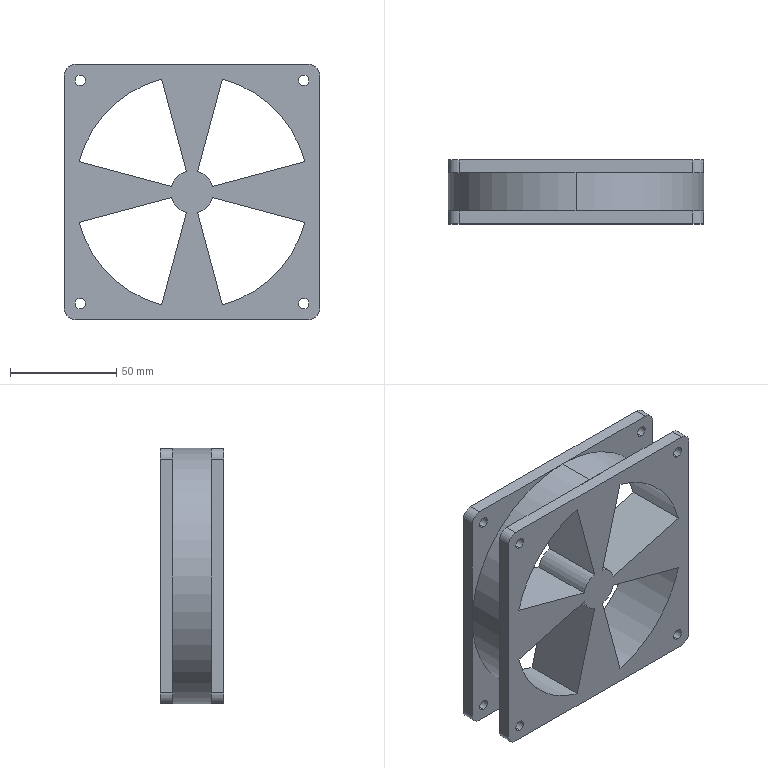Part | SolidWorks | features ICE 3, Extrusion 1, Fillet 1 | 1 solid | 60 faces | box 120 x 30 x 120 mm | volume 191392 mm3 | cylinder 34 | plane 26 | commonest cylinder face diameters 5 x16 10 x8 20 x4 110 x4 120 x2